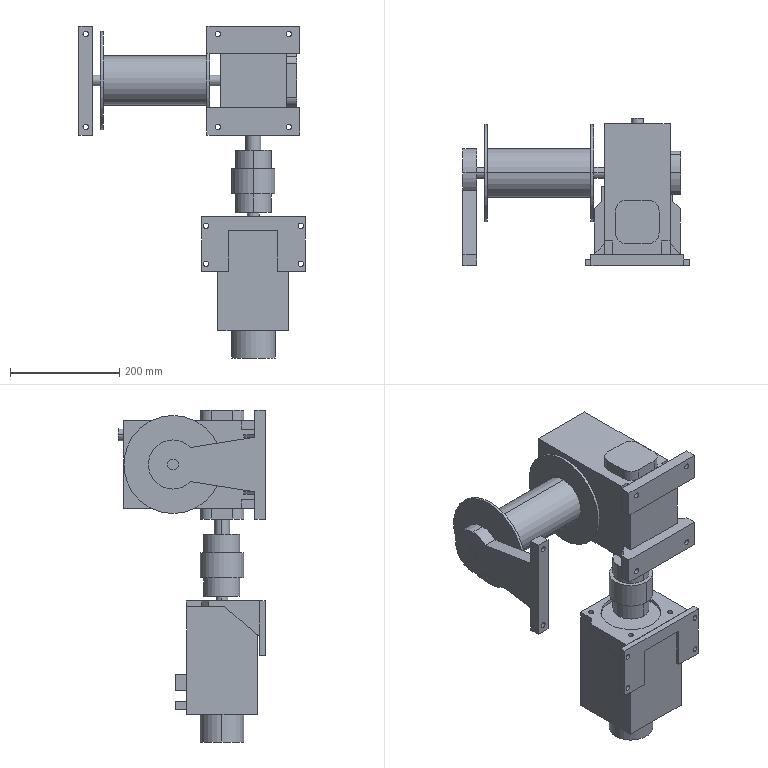Part | SolidWorks | 6 solids | 209 faces | box 415 x 270 x 609 mm | volume 11625644 mm3 | plane 121 | cylinder 88 | commonest cylinder face diameters 10 x28 9.2 x8 40 x8 110 x7 20 x6 22 x6